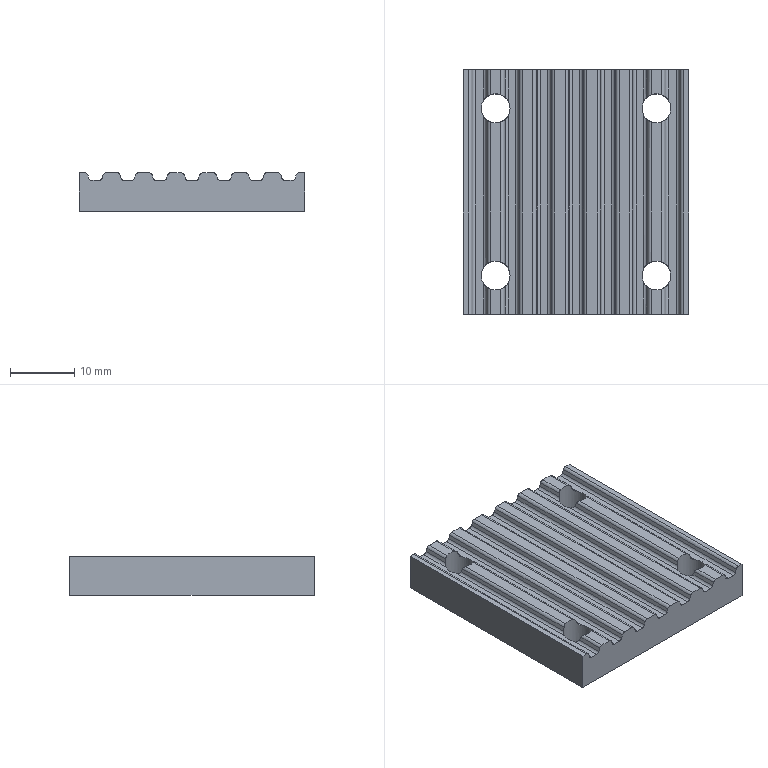Part | NX | 1 solid | 94 faces | box 35 x 38 x 6 mm | volume 6905 mm3 | cylinder 48 | plane 46 | commonest cylinder face diameters 1 x44 4.5 x4